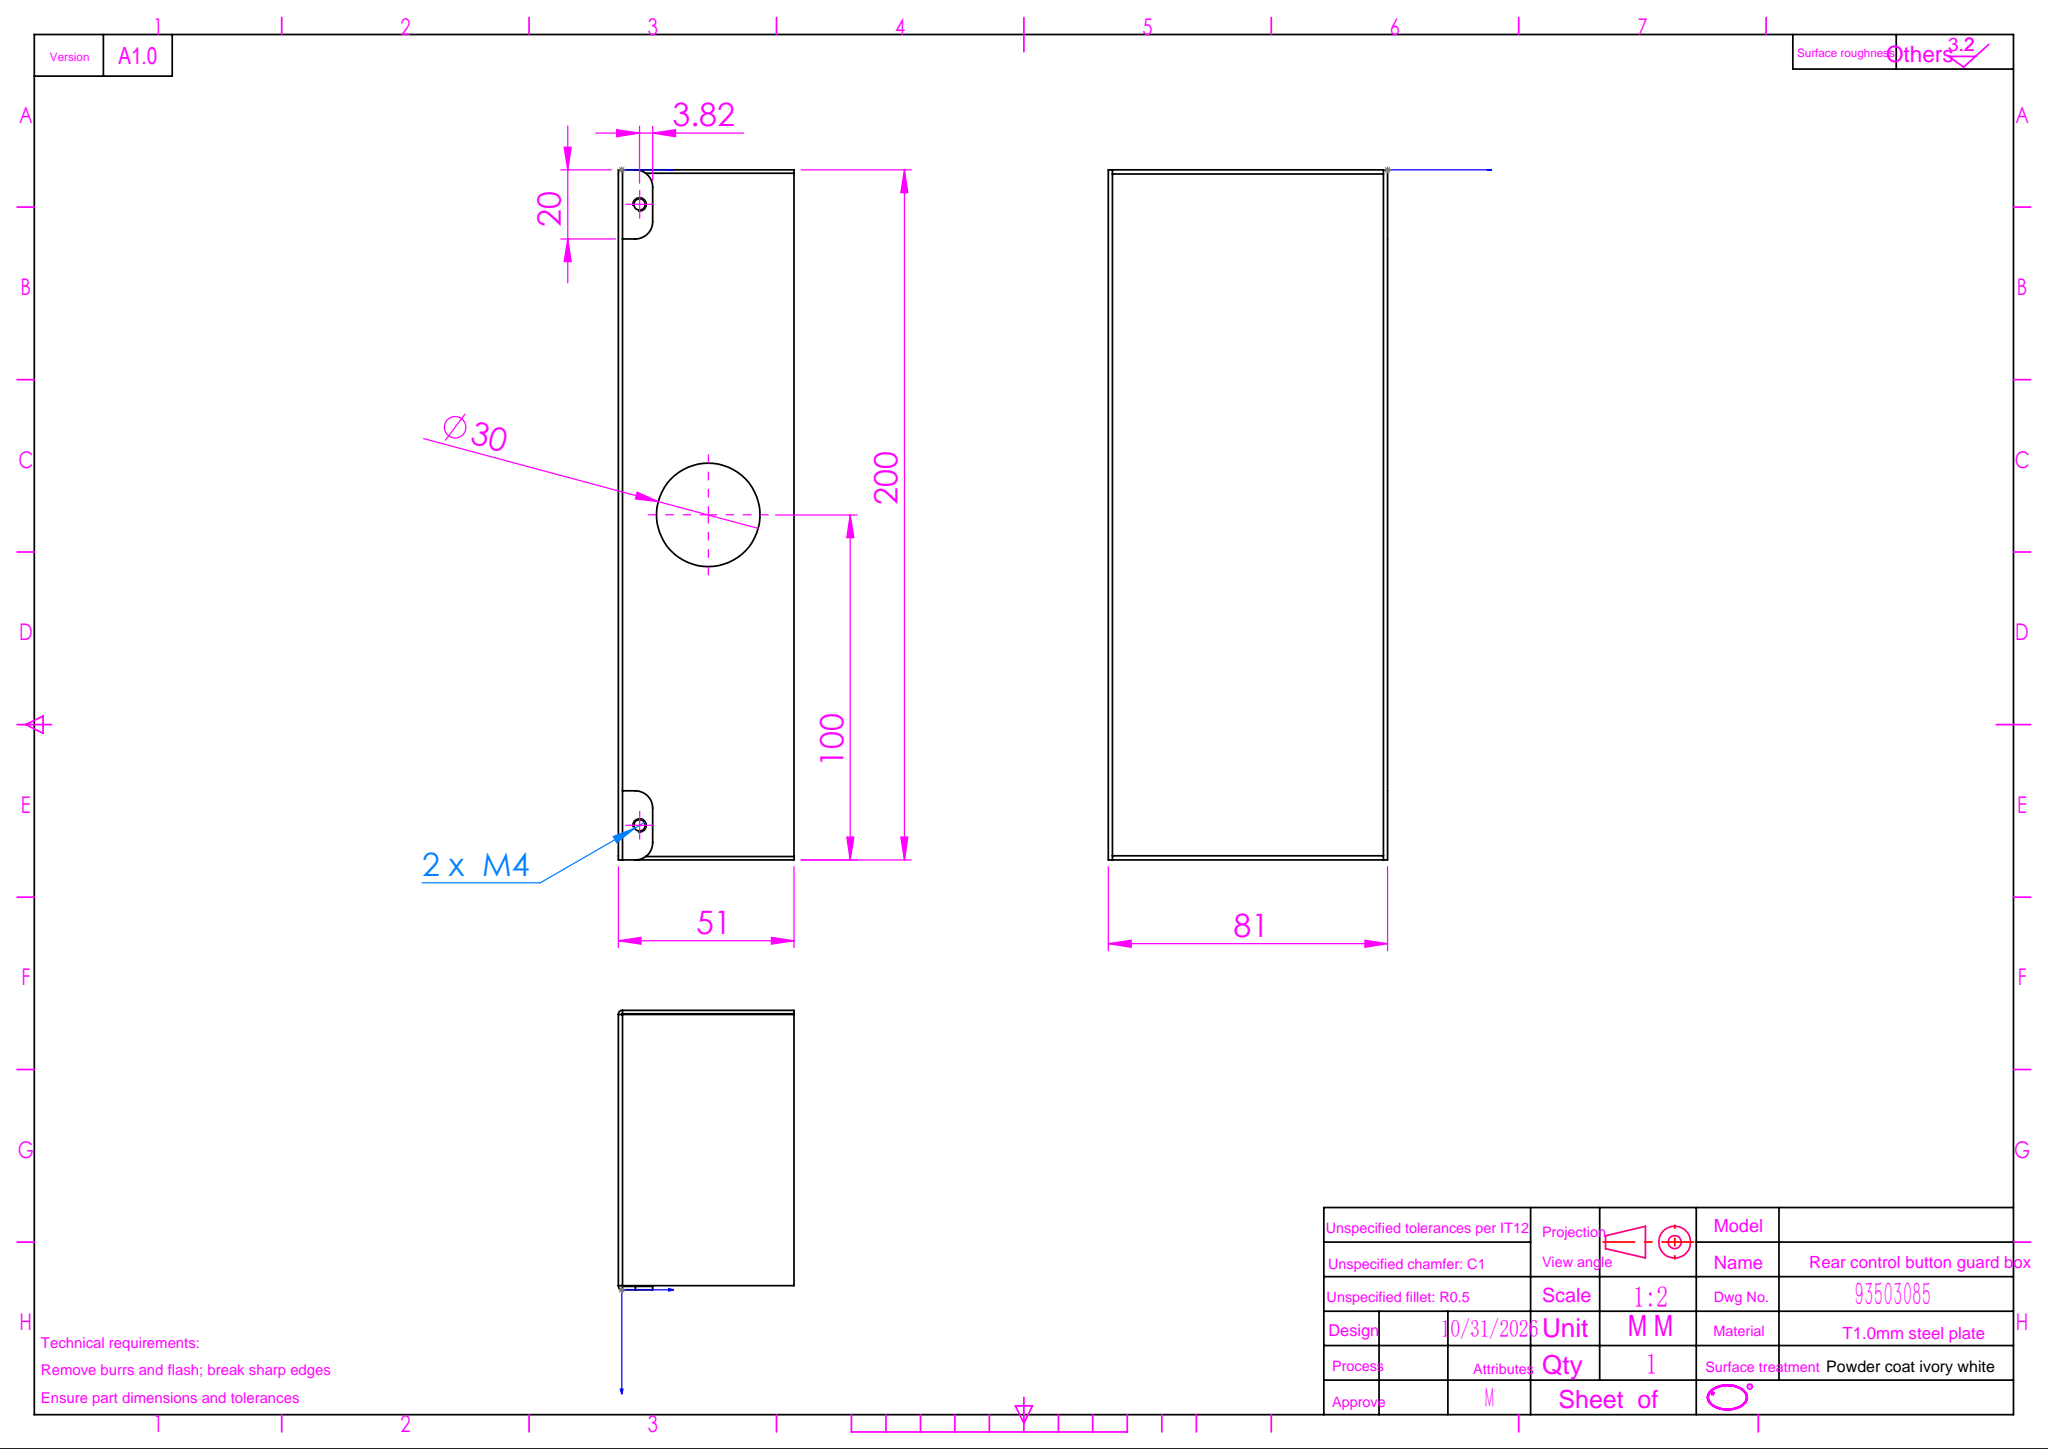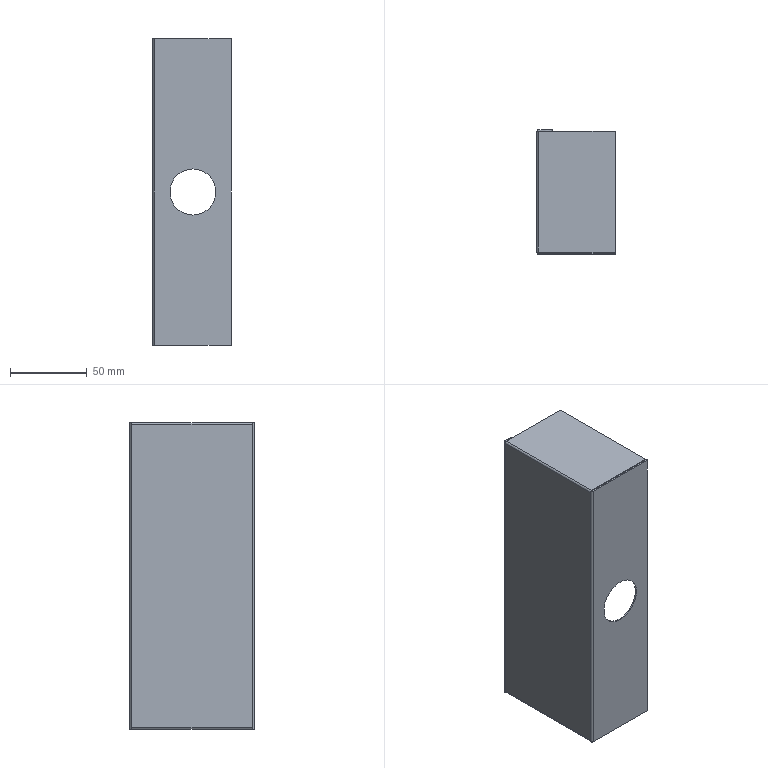Part | SolidWorks | features EdgeFlange 2, ICE 2, 3DProfileFeature 1, Fillet 1, FlatPattern 1, HoleWzd 1, SMBaseFlange 1, SheetMetal 1 | 1 solid | 58 faces | box 51 x 81 x 200 mm | volume 33539 mm3 | plane 40 | cylinder 18 | commonest cylinder face diameters 0.4 x4 2.4 x4 3.3 x4 10 x4 30 x2